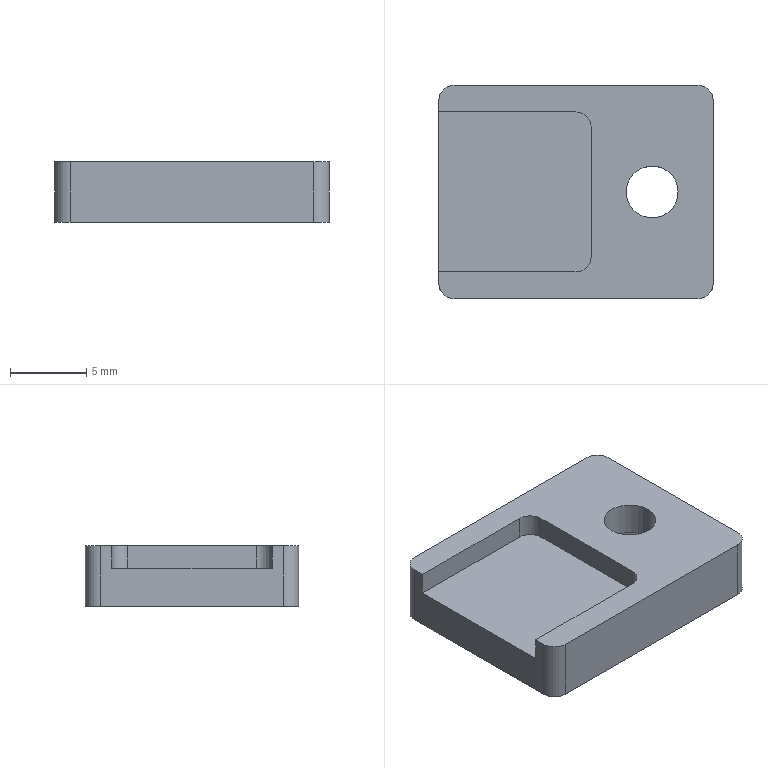Part | SolidWorks | features BaseBody 1 | 1 solid | 20 faces | box 18 x 14 x 4 mm | volume 787.982 mm3 | plane 10 | cylinder 8 | cone 2 | commonest cylinder face diameters 2 x6 3.4 x2
STEP:
#1=CARTESIAN_POINT('',(15.7,7.,1.8));
#2=VERTEX_POINT('',#1);
#3=CARTESIAN_POINT('',(12.3,7.,1.8));
#4=VERTEX_POINT('',#3);
#5=CARTESIAN_POINT('',(14.,7.,1.8));
#6=DIRECTION('',(0.,0.,-1.));
#7=DIRECTION('',(-1.,0.,0.));
#8=AXIS2_PLACEMENT_3D('',#5,#6,#7);
#9=CIRCLE('',#8,1.7);
#10=EDGE_CURVE('',#2,#4,#9,.T.);
#11=ORIENTED_EDGE('',*,*,#10,.F.);
#12=CARTESIAN_POINT('',(17.5,7.,0.));
#13=VERTEX_POINT('',#12);
#14=CARTESIAN_POINT('',(17.5,7.,0.));
#15=DIRECTION('',(0.7071,0.,-0.7071));
#16=VECTOR('',#15,1000.);
#17=LINE('',#14,#16);
#18=EDGE_CURVE('',#2,#13,#17,.T.);
#19=ORIENTED_EDGE('',*,*,#18,.T.);
#20=CARTESIAN_POINT('',(10.5,7.,0.));
#21=VERTEX_POINT('',#20);
#22=CARTESIAN_POINT('',(14.,7.,0.));
#23=DIRECTION('',(0.,0.,1.));
#24=DIRECTION('',(-1.,0.,0.));
#25=AXIS2_PLACEMENT_3D('',#22,#23,#24);
#26=CIRCLE('',#25,3.5);
#27=EDGE_CURVE('',#21,#13,#26,.T.);
#28=ORIENTED_EDGE('',*,*,#27,.F.);
#29=CARTESIAN_POINT('',(10.5,7.,0.));
#30=DIRECTION('',(-0.7071,0.,-0.7071));
#31=VECTOR('',#30,1000.);
#32=LINE('',#29,#31);
#33=EDGE_CURVE('',#4,#21,#32,.T.);
#34=ORIENTED_EDGE('',*,*,#33,.F.);
#35=EDGE_LOOP('',(#11,#19,#28,#34));
#36=FACE_OUTER_BOUND('',#35,.T.);
#37=CARTESIAN_POINT('',(14.,7.,0.));
#38=DIRECTION('',(0.,0.,-1.));
#39=DIRECTION('',(-1.,0.,0.));
#40=AXIS2_PLACEMENT_3D('',#37,#38,#39);
#41=CONICAL_SURFACE('',#40,3.5,0.7854);
#42=ADVANCED_FACE('',(#36),#41,.F.);
#43=CARTESIAN_POINT('',(12.3,7.,4.));
#44=VERTEX_POINT('',#43);
#45=CARTESIAN_POINT('',(15.7,7.,4.));
#46=VERTEX_POINT('',#45);
#47=CARTESIAN_POINT('',(14.,7.,4.));
#48=DIRECTION('',(0.,0.,1.));
#49=DIRECTION('',(-1.,0.,0.));
#50=AXIS2_PLACEMENT_3D('',#47,#48,#49);
#51=CIRCLE('',#50,1.7);
#52=EDGE_CURVE('',#44,#46,#51,.T.);
#53=ORIENTED_EDGE('',*,*,#52,.T.);
#54=CARTESIAN_POINT('',(15.7,7.,0.));
#55=DIRECTION('',(0.,0.,-1.));
#56=VECTOR('',#55,1000.);
#57=LINE('',#54,#56);
#58=EDGE_CURVE('',#46,#2,#57,.T.);
#59=ORIENTED_EDGE('',*,*,#58,.T.);
#60=ORIENTED_EDGE('',*,*,#10,.T.);
#61=CARTESIAN_POINT('',(12.3,7.,0.));
#62=DIRECTION('',(0.,0.,-1.));
#63=VECTOR('',#62,1000.);
#64=LINE('',#61,#63);
#65=EDGE_CURVE('',#44,#4,#64,.T.);
#66=ORIENTED_EDGE('',*,*,#65,.F.);
#67=EDGE_LOOP('',(#53,#59,#60,#66));
#68=FACE_OUTER_BOUND('',#67,.T.);
#69=CARTESIAN_POINT('',(14.,7.,0.));
#70=DIRECTION('',(0.,0.,-1.));
#71=DIRECTION('',(-1.,0.,0.));
#72=AXIS2_PLACEMENT_3D('',#69,#70,#71);
#73=CYLINDRICAL_SURFACE('',#72,1.7);
#74=ADVANCED_FACE('',(#68),#73,.F.);
#75=CARTESIAN_POINT('',(1.,14.,0.));
#76=VERTEX_POINT('',#75);
#77=CARTESIAN_POINT('',(17.,14.,0.));
#78=VERTEX_POINT('',#77);
#79=CARTESIAN_POINT('',(0.,14.,0.));
#80=DIRECTION('',(1.,0.,0.));
#81=VECTOR('',#80,1000.);
#82=LINE('',#79,#81);
#83=EDGE_CURVE('',#76,#78,#82,.T.);
#84=ORIENTED_EDGE('',*,*,#83,.T.);
#85=CARTESIAN_POINT('',(18.,13.,0.));
#86=VERTEX_POINT('',#85);
#87=CARTESIAN_POINT('',(17.,13.,0.));
#88=DIRECTION('',(0.,0.,1.));
#89=DIRECTION('',(-1.,0.,0.));
#90=AXIS2_PLACEMENT_3D('',#87,#88,#89);
#91=CIRCLE('',#90,1.);
#92=EDGE_CURVE('',#86,#78,#91,.T.);
#93=ORIENTED_EDGE('',*,*,#92,.F.);
#94=CARTESIAN_POINT('',(18.,1.,0.));
#95=VERTEX_POINT('',#94);
#96=CARTESIAN_POINT('',(18.,0.,0.));
#97=DIRECTION('',(0.,-1.,0.));
#98=VECTOR('',#97,1000.);
#99=LINE('',#96,#98);
#100=EDGE_CURVE('',#86,#95,#99,.T.);
#101=ORIENTED_EDGE('',*,*,#100,.T.);
#102=CARTESIAN_POINT('',(17.,0.,0.));
#103=VERTEX_POINT('',#102);
#104=CARTESIAN_POINT('',(17.,1.,0.));
#105=DIRECTION('',(0.,0.,1.));
#106=DIRECTION('',(-1.,0.,0.));
#107=AXIS2_PLACEMENT_3D('',#104,#105,#106);
#108=CIRCLE('',#107,1.);
#109=EDGE_CURVE('',#103,#95,#108,.T.);
#110=ORIENTED_EDGE('',*,*,#109,.F.);
#111=CARTESIAN_POINT('',(1.,0.,0.));
#112=VERTEX_POINT('',#111);
#113=CARTESIAN_POINT('',(0.,0.,0.));
#114=DIRECTION('',(-1.,0.,0.));
#115=VECTOR('',#114,1000.);
#116=LINE('',#113,#115);
#117=EDGE_CURVE('',#103,#112,#116,.T.);
#118=ORIENTED_EDGE('',*,*,#117,.T.);
#119=CARTESIAN_POINT('',(0.,1.,0.));
#120=VERTEX_POINT('',#119);
#121=CARTESIAN_POINT('',(1.,1.,0.));
#122=DIRECTION('',(0.,0.,1.));
#123=DIRECTION('',(-1.,0.,0.));
#124=AXIS2_PLACEMENT_3D('',#121,#122,#123);
#125=CIRCLE('',#124,1.);
#126=EDGE_CURVE('',#120,#112,#125,.T.);
#127=ORIENTED_EDGE('',*,*,#126,.F.);
#128=CARTESIAN_POINT('',(0.,13.,0.));
#129=VERTEX_POINT('',#128);
#130=CARTESIAN_POINT('',(0.,0.,0.));
#131=DIRECTION('',(0.,1.,0.));
#132=VECTOR('',#131,1000.);
#133=LINE('',#130,#132);
#134=EDGE_CURVE('',#120,#129,#133,.T.);
#135=ORIENTED_EDGE('',*,*,#134,.T.);
#136=CARTESIAN_POINT('',(1.,13.,0.));
#137=DIRECTION('',(0.,0.,1.));
#138=DIRECTION('',(-1.,0.,0.));
#139=AXIS2_PLACEMENT_3D('',#136,#137,#138);
#140=CIRCLE('',#139,1.);
#141=EDGE_CURVE('',#76,#129,#140,.T.);
#142=ORIENTED_EDGE('',*,*,#141,.F.);
#143=EDGE_LOOP('',(#84,#93,#101,#110,#118,#127,#135,#142));
#144=FACE_OUTER_BOUND('',#143,.T.);
#145=ORIENTED_EDGE('',*,*,#27,.T.);
#146=CARTESIAN_POINT('',(14.,7.,0.));
#147=DIRECTION('',(0.,0.,1.));
#148=DIRECTION('',(-1.,0.,0.));
#149=AXIS2_PLACEMENT_3D('',#146,#147,#148);
#150=CIRCLE('',#149,3.5);
#151=EDGE_CURVE('',#13,#21,#150,.T.);
#152=ORIENTED_EDGE('',*,*,#151,.T.);
#153=EDGE_LOOP('',(#145,#152));
#154=FACE_BOUND('',#153,.T.);
#155=CARTESIAN_POINT('',(0.,0.,0.));
#156=DIRECTION('',(0.,0.,-1.));
#157=DIRECTION('',(-1.,0.,0.));
#158=AXIS2_PLACEMENT_3D('',#155,#156,#157);
#159=PLANE('',#158);
#160=ADVANCED_FACE('',(#144,#154),#159,.T.);
#161=CARTESIAN_POINT('',(1.,14.,4.));
#162=VERTEX_POINT('',#161);
#163=CARTESIAN_POINT('',(1.,14.,4.));
#164=DIRECTION('',(0.,0.,-1.));
#165=VECTOR('',#164,1000.);
#166=LINE('',#163,#165);
#167=EDGE_CURVE('',#162,#76,#166,.T.);
#168=ORIENTED_EDGE('',*,*,#167,.F.);
#169=CARTESIAN_POINT('',(17.,14.,4.));
#170=VERTEX_POINT('',#169);
#171=CARTESIAN_POINT('',(0.,14.,4.));
#172=DIRECTION('',(-1.,0.,0.));
#173=VECTOR('',#172,1000.);
#174=LINE('',#171,#173);
#175=EDGE_CURVE('',#170,#162,#174,.T.);
#176=ORIENTED_EDGE('',*,*,#175,.F.);
#177=CARTESIAN_POINT('',(17.,14.,4.));
#178=DIRECTION('',(0.,0.,1.));
#179=VECTOR('',#178,1000.);
#180=LINE('',#177,#179);
#181=EDGE_CURVE('',#78,#170,#180,.T.);
#182=ORIENTED_EDGE('',*,*,#181,.F.);
#183=ORIENTED_EDGE('',*,*,#83,.F.);
#184=EDGE_LOOP('',(#168,#176,#182,#183));
#185=FACE_OUTER_BOUND('',#184,.T.);
#186=CARTESIAN_POINT('',(0.,14.,4.));
#187=DIRECTION('',(0.,-1.,0.));
#188=DIRECTION('',(0.,0.,-1.));
#189=AXIS2_PLACEMENT_3D('',#186,#187,#188);
#190=PLANE('',#189);
#191=ADVANCED_FACE('',(#185),#190,.F.);
#192=CARTESIAN_POINT('',(0.,1.,4.));
#193=VERTEX_POINT('',#192);
#194=CARTESIAN_POINT('',(0.,1.,4.));
#195=DIRECTION('',(0.,0.,-1.));
#196=VECTOR('',#195,1000.);
#197=LINE('',#194,#196);
#198=EDGE_CURVE('',#193,#120,#197,.T.);
#199=ORIENTED_EDGE('',*,*,#198,.F.);
#200=CARTESIAN_POINT('',(0.,1.75,4.));
#201=VERTEX_POINT('',#200);
#202=CARTESIAN_POINT('',(0.,0.,4.));
#203=DIRECTION('',(0.,-1.,0.));
#204=VECTOR('',#203,1000.);
#205=LINE('',#202,#204);
#206=EDGE_CURVE('',#201,#193,#205,.T.);
#207=ORIENTED_EDGE('',*,*,#206,.F.);
#208=CARTESIAN_POINT('',(0.,1.75,2.5));
#209=VERTEX_POINT('',#208);
#210=CARTESIAN_POINT('',(0.,1.75,2.5));
#211=DIRECTION('',(0.,0.,-1.));
#212=VECTOR('',#211,1000.);
#213=LINE('',#210,#212);
#214=EDGE_CURVE('',#201,#209,#213,.T.);
#215=ORIENTED_EDGE('',*,*,#214,.T.);
#216=CARTESIAN_POINT('',(0.,12.25,2.5));
#217=VERTEX_POINT('',#216);
#218=CARTESIAN_POINT('',(0.,0.,2.5));
#219=DIRECTION('',(0.,-1.,0.));
#220=VECTOR('',#219,1000.);
#221=LINE('',#218,#220);
#222=EDGE_CURVE('',#217,#209,#221,.T.);
#223=ORIENTED_EDGE('',*,*,#222,.F.);
#224=CARTESIAN_POINT('',(0.,12.25,4.));
#225=VERTEX_POINT('',#224);
#226=CARTESIAN_POINT('',(0.,12.25,2.5));
#227=DIRECTION('',(0.,0.,1.));
#228=VECTOR('',#227,1000.);
#229=LINE('',#226,#228);
#230=EDGE_CURVE('',#217,#225,#229,.T.);
#231=ORIENTED_EDGE('',*,*,#230,.T.);
#232=CARTESIAN_POINT('',(0.,13.,4.));
#233=VERTEX_POINT('',#232);
#234=CARTESIAN_POINT('',(0.,0.,4.));
#235=DIRECTION('',(0.,-1.,0.));
#236=VECTOR('',#235,1000.);
#237=LINE('',#234,#236);
#238=EDGE_CURVE('',#233,#225,#237,.T.);
#239=ORIENTED_EDGE('',*,*,#238,.F.);
#240=CARTESIAN_POINT('',(0.,13.,4.));
#241=DIRECTION('',(0.,0.,1.));
#242=VECTOR('',#241,1000.);
#243=LINE('',#240,#242);
#244=EDGE_CURVE('',#129,#233,#243,.T.);
#245=ORIENTED_EDGE('',*,*,#244,.F.);
#246=ORIENTED_EDGE('',*,*,#134,.F.);
#247=EDGE_LOOP('',(#199,#207,#215,#223,#231,#239,#245,#246));
#248=FACE_OUTER_BOUND('',#247,.T.);
#249=CARTESIAN_POINT('',(0.,0.,4.));
#250=DIRECTION('',(1.,0.,0.));
#251=DIRECTION('',(0.,0.,-1.));
#252=AXIS2_PLACEMENT_3D('',#249,#250,#251);
#253=PLANE('',#252);
#254=ADVANCED_FACE('',(#248),#253,.F.);
#255=CARTESIAN_POINT('',(17.,0.,4.));
#256=VERTEX_POINT('',#255);
#257=CARTESIAN_POINT('',(17.,0.,4.));
#258=DIRECTION('',(0.,0.,-1.));
#259=VECTOR('',#258,1000.);
#260=LINE('',#257,#259);
#261=EDGE_CURVE('',#256,#103,#260,.T.);
#262=ORIENTED_EDGE('',*,*,#261,.F.);
#263=CARTESIAN_POINT('',(1.,0.,4.));
#264=VERTEX_POINT('',#263);
#265=CARTESIAN_POINT('',(0.,0.,4.));
#266=DIRECTION('',(1.,0.,0.));
#267=VECTOR('',#266,1000.);
#268=LINE('',#265,#267);
#269=EDGE_CURVE('',#264,#256,#268,.T.);
#270=ORIENTED_EDGE('',*,*,#269,.F.);
#271=CARTESIAN_POINT('',(1.,0.,4.));
#272=DIRECTION('',(0.,0.,1.));
#273=VECTOR('',#272,1000.);
#274=LINE('',#271,#273);
#275=EDGE_CURVE('',#112,#264,#274,.T.);
#276=ORIENTED_EDGE('',*,*,#275,.F.);
#277=ORIENTED_EDGE('',*,*,#117,.F.);
#278=EDGE_LOOP('',(#262,#270,#276,#277));
#279=FACE_OUTER_BOUND('',#278,.T.);
#280=CARTESIAN_POINT('',(0.,0.,4.));
#281=DIRECTION('',(0.,1.,0.));
#282=DIRECTION('',(0.,0.,1.));
#283=AXIS2_PLACEMENT_3D('',#280,#281,#282);
#284=PLANE('',#283);
#285=ADVANCED_FACE('',(#279),#284,.F.);
#286=CARTESIAN_POINT('',(18.,1.,4.));
#287=VERTEX_POINT('',#286);
#288=CARTESIAN_POINT('',(18.,1.,4.));
#289=DIRECTION('',(0.,0.,1.));
#290=VECTOR('',#289,1000.);
#291=LINE('',#288,#290);
#292=EDGE_CURVE('',#95,#287,#291,.T.);
#293=ORIENTED_EDGE('',*,*,#292,.F.);
#294=ORIENTED_EDGE('',*,*,#100,.F.);
#295=CARTESIAN_POINT('',(18.,13.,4.));
#296=VERTEX_POINT('',#295);
#297=CARTESIAN_POINT('',(18.,13.,4.));
#298=DIRECTION('',(0.,0.,-1.));
#299=VECTOR('',#298,1000.);
#300=LINE('',#297,#299);
#301=EDGE_CURVE('',#296,#86,#300,.T.);
#302=ORIENTED_EDGE('',*,*,#301,.F.);
#303=CARTESIAN_POINT('',(18.,0.,4.));
#304=DIRECTION('',(0.,1.,0.));
#305=VECTOR('',#304,1000.);
#306=LINE('',#303,#305);
#307=EDGE_CURVE('',#287,#296,#306,.T.);
#308=ORIENTED_EDGE('',*,*,#307,.F.);
#309=EDGE_LOOP('',(#293,#294,#302,#308));
#310=FACE_OUTER_BOUND('',#309,.T.);
#311=CARTESIAN_POINT('',(18.,0.,4.));
#312=DIRECTION('',(-1.,0.,0.));
#313=DIRECTION('',(0.,0.,1.));
#314=AXIS2_PLACEMENT_3D('',#311,#312,#313);
#315=PLANE('',#314);
#316=ADVANCED_FACE('',(#310),#315,.F.);
#317=ORIENTED_EDGE('',*,*,#18,.F.);
#318=CARTESIAN_POINT('',(14.,7.,1.8));
#319=DIRECTION('',(0.,0.,-1.));
#320=DIRECTION('',(-1.,0.,0.));
#321=AXIS2_PLACEMENT_3D('',#318,#319,#320);
#322=CIRCLE('',#321,1.7);
#323=EDGE_CURVE('',#4,#2,#322,.T.);
#324=ORIENTED_EDGE('',*,*,#323,.F.);
#325=ORIENTED_EDGE('',*,*,#33,.T.);
#326=ORIENTED_EDGE('',*,*,#151,.F.);
#327=EDGE_LOOP('',(#317,#324,#325,#326));
#328=FACE_OUTER_BOUND('',#327,.T.);
#329=CARTESIAN_POINT('',(14.,7.,0.));
#330=DIRECTION('',(0.,0.,-1.));
#331=DIRECTION('',(-1.,0.,0.));
#332=AXIS2_PLACEMENT_3D('',#329,#330,#331);
#333=CONICAL_SURFACE('',#332,3.5,0.7854);
#334=ADVANCED_FACE('',(#328),#333,.F.);
#335=ORIENTED_EDGE('',*,*,#141,.T.);
#336=ORIENTED_EDGE('',*,*,#244,.T.);
#337=CARTESIAN_POINT('',(1.,13.,4.));
#338=DIRECTION('',(0.,0.,-1.));
#339=DIRECTION('',(-1.,0.,0.));
#340=AXIS2_PLACEMENT_3D('',#337,#338,#339);
#341=CIRCLE('',#340,1.);
#342=EDGE_CURVE('',#233,#162,#341,.T.);
#343=ORIENTED_EDGE('',*,*,#342,.T.);
#344=ORIENTED_EDGE('',*,*,#167,.T.);
#345=EDGE_LOOP('',(#335,#336,#343,#344));
#346=FACE_OUTER_BOUND('',#345,.T.);
#347=CARTESIAN_POINT('',(1.,13.,4.));
#348=DIRECTION('',(0.,0.,-1.));
#349=DIRECTION('',(-1.,0.,0.));
#350=AXIS2_PLACEMENT_3D('',#347,#348,#349);
#351=CYLINDRICAL_SURFACE('',#350,1.);
#352=ADVANCED_FACE('',(#346),#351,.T.);
#353=CARTESIAN_POINT('',(17.,1.,4.));
#354=DIRECTION('',(0.,0.,-1.));
#355=DIRECTION('',(-1.,0.,0.));
#356=AXIS2_PLACEMENT_3D('',#353,#354,#355);
#357=CIRCLE('',#356,1.);
#358=EDGE_CURVE('',#287,#256,#357,.T.);
#359=ORIENTED_EDGE('',*,*,#358,.F.);
#360=ORIENTED_EDGE('',*,*,#307,.T.);
#361=CARTESIAN_POINT('',(17.,13.,4.));
#362=DIRECTION('',(0.,0.,-1.));
#363=DIRECTION('',(-1.,0.,0.));
#364=AXIS2_PLACEMENT_3D('',#361,#362,#363);
#365=CIRCLE('',#364,1.);
#366=EDGE_CURVE('',#170,#296,#365,.T.);
#367=ORIENTED_EDGE('',*,*,#366,.F.);
#368=ORIENTED_EDGE('',*,*,#175,.T.);
#369=ORIENTED_EDGE('',*,*,#342,.F.);
#370=ORIENTED_EDGE('',*,*,#238,.T.);
#371=CARTESIAN_POINT('',(9.,12.25,4.));
#372=VERTEX_POINT('',#371);
#373=CARTESIAN_POINT('',(0.,12.25,4.));
#374=DIRECTION('',(-1.,0.,0.));
#375=VECTOR('',#374,1000.);
#376=LINE('',#373,#375);
#377=EDGE_CURVE('',#372,#225,#376,.T.);
#378=ORIENTED_EDGE('',*,*,#377,.F.);
#379=CARTESIAN_POINT('',(10.,11.25,4.));
#380=VERTEX_POINT('',#379);
#381=CARTESIAN_POINT('',(9.,11.25,4.));
#382=DIRECTION('',(0.,0.,1.));
#383=DIRECTION('',(-1.,0.,0.));
#384=AXIS2_PLACEMENT_3D('',#381,#382,#383);
#385=CIRCLE('',#384,1.);
#386=EDGE_CURVE('',#380,#372,#385,.T.);
#387=ORIENTED_EDGE('',*,*,#386,.F.);
#388=CARTESIAN_POINT('',(10.,2.75,4.));
#389=VERTEX_POINT('',#388);
#390=CARTESIAN_POINT('',(10.,0.,4.));
#391=DIRECTION('',(0.,1.,0.));
#392=VECTOR('',#391,1000.);
#393=LINE('',#390,#392);
#394=EDGE_CURVE('',#389,#380,#393,.T.);
#395=ORIENTED_EDGE('',*,*,#394,.F.);
#396=CARTESIAN_POINT('',(9.,1.75,4.));
#397=VERTEX_POINT('',#396);
#398=CARTESIAN_POINT('',(9.,2.75,4.));
#399=DIRECTION('',(0.,0.,1.));
#400=DIRECTION('',(-1.,0.,0.));
#401=AXIS2_PLACEMENT_3D('',#398,#399,#400);
#402=CIRCLE('',#401,1.);
#403=EDGE_CURVE('',#397,#389,#402,.T.);
#404=ORIENTED_EDGE('',*,*,#403,.F.);
#405=CARTESIAN_POINT('',(0.,1.75,4.));
#406=DIRECTION('',(1.,0.,0.));
#407=VECTOR('',#406,1000.);
#408=LINE('',#405,#407);
#409=EDGE_CURVE('',#201,#397,#408,.T.);
#410=ORIENTED_EDGE('',*,*,#409,.F.);
#411=ORIENTED_EDGE('',*,*,#206,.T.);
#412=CARTESIAN_POINT('',(1.,1.,4.));
#413=DIRECTION('',(0.,0.,-1.));
#414=DIRECTION('',(-1.,0.,0.));
#415=AXIS2_PLACEMENT_3D('',#412,#413,#414);
#416=CIRCLE('',#415,1.);
#417=EDGE_CURVE('',#264,#193,#416,.T.);
#418=ORIENTED_EDGE('',*,*,#417,.F.);
#419=ORIENTED_EDGE('',*,*,#269,.T.);
#420=EDGE_LOOP('',(#359,#360,#367,#368,#369,#370,#378,#387,#395,#404,#410,#411,#418,#419));
#421=FACE_OUTER_BOUND('',#420,.T.);
#422=ORIENTED_EDGE('',*,*,#52,.F.);
#423=CARTESIAN_POINT('',(14.,7.,4.));
#424=DIRECTION('',(0.,0.,1.));
#425=DIRECTION('',(-1.,0.,0.));
#426=AXIS2_PLACEMENT_3D('',#423,#424,#425);
#427=CIRCLE('',#426,1.7);
#428=EDGE_CURVE('',#46,#44,#427,.T.);
#429=ORIENTED_EDGE('',*,*,#428,.F.);
#430=EDGE_LOOP('',(#422,#429));
#431=FACE_BOUND('',#430,.T.);
#432=CARTESIAN_POINT('',(0.,0.,4.));
#433=DIRECTION('',(0.,0.,-1.));
#434=DIRECTION('',(-1.,0.,0.));
#435=AXIS2_PLACEMENT_3D('',#432,#433,#434);
#436=PLANE('',#435);
#437=ADVANCED_FACE('',(#421,#431),#436,.F.);
#438=ORIENTED_EDGE('',*,*,#92,.T.);
#439=ORIENTED_EDGE('',*,*,#181,.T.);
#440=ORIENTED_EDGE('',*,*,#366,.T.);
#441=ORIENTED_EDGE('',*,*,#301,.T.);
#442=EDGE_LOOP('',(#438,#439,#440,#441));
#443=FACE_OUTER_BOUND('',#442,.T.);
#444=CARTESIAN_POINT('',(17.,13.,4.));
#445=DIRECTION('',(0.,0.,-1.));
#446=DIRECTION('',(-1.,0.,0.));
#447=AXIS2_PLACEMENT_3D('',#444,#445,#446);
#448=CYLINDRICAL_SURFACE('',#447,1.);
#449=ADVANCED_FACE('',(#443),#448,.T.);
#450=ORIENTED_EDGE('',*,*,#126,.T.);
#451=ORIENTED_EDGE('',*,*,#275,.T.);
#452=ORIENTED_EDGE('',*,*,#417,.T.);
#453=ORIENTED_EDGE('',*,*,#198,.T.);
#454=EDGE_LOOP('',(#450,#451,#452,#453));
#455=FACE_OUTER_BOUND('',#454,.T.);
#456=CARTESIAN_POINT('',(1.,1.,4.));
#457=DIRECTION('',(0.,0.,-1.));
#458=DIRECTION('',(-1.,0.,0.));
#459=AXIS2_PLACEMENT_3D('',#456,#457,#458);
#460=CYLINDRICAL_SURFACE('',#459,1.);
#461=ADVANCED_FACE('',(#455),#460,.T.);
#462=CARTESIAN_POINT('',(9.,12.25,2.5));
#463=VERTEX_POINT('',#462);
#464=CARTESIAN_POINT('',(0.,12.25,2.5));
#465=DIRECTION('',(-1.,0.,0.));
#466=VECTOR('',#465,1000.);
#467=LINE('',#464,#466);
#468=EDGE_CURVE('',#463,#217,#467,.T.);
#469=ORIENTED_EDGE('',*,*,#468,.T.);
#470=ORIENTED_EDGE('',*,*,#222,.T.);
#471=CARTESIAN_POINT('',(9.,1.75,2.5));
#472=VERTEX_POINT('',#471);
#473=CARTESIAN_POINT('',(0.,1.75,2.5));
#474=DIRECTION('',(1.,0.,0.));
#475=VECTOR('',#474,1000.);
#476=LINE('',#473,#475);
#477=EDGE_CURVE('',#209,#472,#476,.T.);
#478=ORIENTED_EDGE('',*,*,#477,.T.);
#479=CARTESIAN_POINT('',(10.,2.75,2.5));
#480=VERTEX_POINT('',#479);
#481=CARTESIAN_POINT('',(9.,2.75,2.5));
#482=DIRECTION('',(0.,0.,1.));
#483=DIRECTION('',(-1.,0.,0.));
#484=AXIS2_PLACEMENT_3D('',#481,#482,#483);
#485=CIRCLE('',#484,1.);
#486=EDGE_CURVE('',#472,#480,#485,.T.);
#487=ORIENTED_EDGE('',*,*,#486,.T.);
#488=CARTESIAN_POINT('',(10.,11.25,2.5));
#489=VERTEX_POINT('',#488);
#490=CARTESIAN_POINT('',(10.,0.,2.5));
#491=DIRECTION('',(0.,1.,0.));
#492=VECTOR('',#491,1000.);
#493=LINE('',#490,#492);
#494=EDGE_CURVE('',#480,#489,#493,.T.);
#495=ORIENTED_EDGE('',*,*,#494,.T.);
#496=CARTESIAN_POINT('',(9.,11.25,2.5));
#497=DIRECTION('',(0.,0.,1.));
#498=DIRECTION('',(-1.,0.,0.));
#499=AXIS2_PLACEMENT_3D('',#496,#497,#498);
#500=CIRCLE('',#499,1.);
#501=EDGE_CURVE('',#489,#463,#500,.T.);
#502=ORIENTED_EDGE('',*,*,#501,.T.);
#503=EDGE_LOOP('',(#469,#470,#478,#487,#495,#502));
#504=FACE_OUTER_BOUND('',#503,.T.);
#505=CARTESIAN_POINT('',(0.,0.,2.5));
#506=DIRECTION('',(0.,0.,1.));
#507=DIRECTION('',(1.,0.,0.));
#508=AXIS2_PLACEMENT_3D('',#505,#506,#507);
#509=PLANE('',#508);
#510=ADVANCED_FACE('',(#504),#509,.T.);
#511=ORIENTED_EDGE('',*,*,#109,.T.);
#512=ORIENTED_EDGE('',*,*,#292,.T.);
#513=ORIENTED_EDGE('',*,*,#358,.T.);
#514=ORIENTED_EDGE('',*,*,#261,.T.);
#515=EDGE_LOOP('',(#511,#512,#513,#514));
#516=FACE_OUTER_BOUND('',#515,.T.);
#517=CARTESIAN_POINT('',(17.,1.,4.));
#518=DIRECTION('',(0.,0.,-1.));
#519=DIRECTION('',(-1.,0.,0.));
#520=AXIS2_PLACEMENT_3D('',#517,#518,#519);
#521=CYLINDRICAL_SURFACE('',#520,1.);
#522=ADVANCED_FACE('',(#516),#521,.T.);
#523=ORIENTED_EDGE('',*,*,#58,.F.);
#524=ORIENTED_EDGE('',*,*,#428,.T.);
#525=ORIENTED_EDGE('',*,*,#65,.T.);
#526=ORIENTED_EDGE('',*,*,#323,.T.);
#527=EDGE_LOOP('',(#523,#524,#525,#526));
#528=FACE_OUTER_BOUND('',#527,.T.);
#529=CARTESIAN_POINT('',(14.,7.,0.));
#530=DIRECTION('',(0.,0.,-1.));
#531=DIRECTION('',(-1.,0.,0.));
#532=AXIS2_PLACEMENT_3D('',#529,#530,#531);
#533=CYLINDRICAL_SURFACE('',#532,1.7);
#534=ADVANCED_FACE('',(#528),#533,.F.);
#535=CARTESIAN_POINT('',(9.,12.25,2.5));
#536=DIRECTION('',(0.,0.,-1.));
#537=VECTOR('',#536,1000.);
#538=LINE('',#535,#537);
#539=EDGE_CURVE('',#372,#463,#538,.T.);
#540=ORIENTED_EDGE('',*,*,#539,.F.);
#541=ORIENTED_EDGE('',*,*,#377,.T.);
#542=ORIENTED_EDGE('',*,*,#230,.F.);
#543=ORIENTED_EDGE('',*,*,#468,.F.);
#544=EDGE_LOOP('',(#540,#541,#542,#543));
#545=FACE_OUTER_BOUND('',#544,.T.);
#546=CARTESIAN_POINT('',(0.,12.25,2.5));
#547=DIRECTION('',(0.,1.,0.));
#548=DIRECTION('',(-1.,0.,0.));
#549=AXIS2_PLACEMENT_3D('',#546,#547,#548);
#550=PLANE('',#549);
#551=ADVANCED_FACE('',(#545),#550,.F.);
#552=CARTESIAN_POINT('',(10.,11.25,2.5));
#553=DIRECTION('',(0.,0.,-1.));
#554=VECTOR('',#553,1000.);
#555=LINE('',#552,#554);
#556=EDGE_CURVE('',#380,#489,#555,.T.);
#557=ORIENTED_EDGE('',*,*,#556,.F.);
#558=ORIENTED_EDGE('',*,*,#386,.T.);
#559=ORIENTED_EDGE('',*,*,#539,.T.);
#560=ORIENTED_EDGE('',*,*,#501,.F.);
#561=EDGE_LOOP('',(#557,#558,#559,#560));
#562=FACE_OUTER_BOUND('',#561,.T.);
#563=CARTESIAN_POINT('',(9.,11.25,2.5));
#564=DIRECTION('',(0.,0.,-1.));
#565=DIRECTION('',(-1.,0.,0.));
#566=AXIS2_PLACEMENT_3D('',#563,#564,#565);
#567=CYLINDRICAL_SURFACE('',#566,1.);
#568=ADVANCED_FACE('',(#562),#567,.F.);
#569=CARTESIAN_POINT('',(10.,2.75,2.5));
#570=DIRECTION('',(0.,0.,-1.));
#571=VECTOR('',#570,1000.);
#572=LINE('',#569,#571);
#573=EDGE_CURVE('',#389,#480,#572,.T.);
#574=ORIENTED_EDGE('',*,*,#573,.F.);
#575=ORIENTED_EDGE('',*,*,#394,.T.);
#576=ORIENTED_EDGE('',*,*,#556,.T.);
#577=ORIENTED_EDGE('',*,*,#494,.F.);
#578=EDGE_LOOP('',(#574,#575,#576,#577));
#579=FACE_OUTER_BOUND('',#578,.T.);
#580=CARTESIAN_POINT('',(10.,12.25,2.5));
#581=DIRECTION('',(1.,0.,0.));
#582=DIRECTION('',(0.,1.,0.));
#583=AXIS2_PLACEMENT_3D('',#580,#581,#582);
#584=PLANE('',#583);
#585=ADVANCED_FACE('',(#579),#584,.F.);
#586=CARTESIAN_POINT('',(9.,1.75,2.5));
#587=DIRECTION('',(0.,0.,-1.));
#588=VECTOR('',#587,1000.);
#589=LINE('',#586,#588);
#590=EDGE_CURVE('',#397,#472,#589,.T.);
#591=ORIENTED_EDGE('',*,*,#590,.F.);
#592=ORIENTED_EDGE('',*,*,#403,.T.);
#593=ORIENTED_EDGE('',*,*,#573,.T.);
#594=ORIENTED_EDGE('',*,*,#486,.F.);
#595=EDGE_LOOP('',(#591,#592,#593,#594));
#596=FACE_OUTER_BOUND('',#595,.T.);
#597=CARTESIAN_POINT('',(9.,2.75,2.5));
#598=DIRECTION('',(0.,0.,-1.));
#599=DIRECTION('',(-1.,0.,0.));
#600=AXIS2_PLACEMENT_3D('',#597,#598,#599);
#601=CYLINDRICAL_SURFACE('',#600,1.);
#602=ADVANCED_FACE('',(#596),#601,.F.);
#603=ORIENTED_EDGE('',*,*,#590,.T.);
#604=ORIENTED_EDGE('',*,*,#477,.F.);
#605=ORIENTED_EDGE('',*,*,#214,.F.);
#606=ORIENTED_EDGE('',*,*,#409,.T.);
#607=EDGE_LOOP('',(#603,#604,#605,#606));
#608=FACE_OUTER_BOUND('',#607,.T.);
#609=CARTESIAN_POINT('',(0.,1.75,2.5));
#610=DIRECTION('',(0.,-1.,0.));
#611=DIRECTION('',(0.,0.,-1.));
#612=AXIS2_PLACEMENT_3D('',#609,#610,#611);
#613=PLANE('',#612);
#614=ADVANCED_FACE('',(#608),#613,.F.);
#615=CLOSED_SHELL('',(#42,#74,#160,#191,#254,#285,#316,#334,#352,#437,#449,#461,#510,#522,#534,#551,#568,#585,#602,#614));
#616=MANIFOLD_SOLID_BREP('',#615);
#617=CARTESIAN_POINT('',(0.,0.,0.));
#618=DIRECTION('',(0.,0.,1.));
#619=DIRECTION('',(1.,0.,0.));
#620=AXIS2_PLACEMENT_3D('',#617,#618,#619);
#621=(LENGTH_UNIT()NAMED_UNIT(*)SI_UNIT(.MILLI.,.METRE.));
#622=UNCERTAINTY_MEASURE_WITH_UNIT(LENGTH_MEASURE(0.00001),#621,'','');
#623=(NAMED_UNIT(*)PLANE_ANGLE_UNIT()SI_UNIT($,.RADIAN.));
#624=(NAMED_UNIT(*)SI_UNIT($,.STERADIAN.)SOLID_ANGLE_UNIT());
#625=(GEOMETRIC_REPRESENTATION_CONTEXT(3)GLOBAL_UNCERTAINTY_ASSIGNED_CONTEXT((#622))GLOBAL_UNIT_ASSIGNED_CONTEXT((#621,#623,#624))REPRESENTATION_CONTEXT('',''));
#626=ADVANCED_BREP_SHAPE_REPRESENTATION('',(#616,#620),#625);